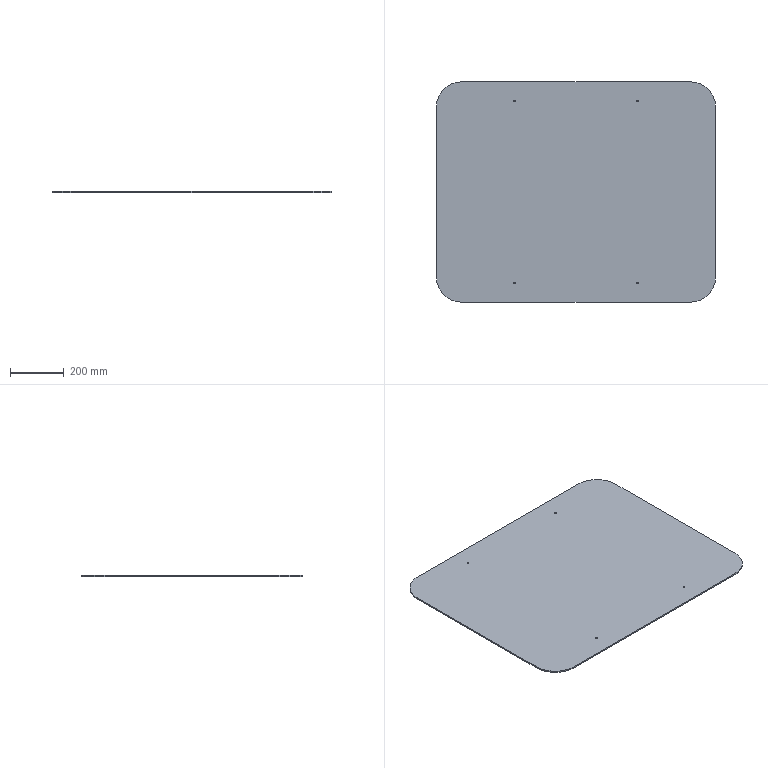Part | NX | features BREP 1 | 1 solid | 14 faces | box 1040 x 820 x 5 mm | volume 4224601 mm3 | cylinder 8 | plane 6 | commonest cylinder face diameters 6.5 x4 190 x4
STEP:
#1=CARTESIAN_POINT('',(232.75,338.5,-5.));
#2=VERTEX_POINT('',#1);
#3=CARTESIAN_POINT('',(229.5,338.5,-5.));
#4=DIRECTION('',(0.,0.,-1.));
#5=DIRECTION('',(1.,0.,0.));
#6=AXIS2_PLACEMENT_3D('',#3,#4,#5);
#7=CIRCLE('',#6,3.25);
#8=EDGE_CURVE('',#2,#2,#7,.T.);
#9=ORIENTED_EDGE('',*,*,#8,.T.);
#10=EDGE_LOOP('',(#9));
#11=FACE_BOUND('',#10,.T.);
#12=CARTESIAN_POINT('',(226.25,338.5,0.));
#13=VERTEX_POINT('',#12);
#14=CARTESIAN_POINT('',(229.5,338.5,0.));
#15=DIRECTION('',(0.,0.,-1.));
#16=DIRECTION('',(-1.,0.,0.));
#17=AXIS2_PLACEMENT_3D('',#14,#15,#16);
#18=CIRCLE('',#17,3.25);
#19=EDGE_CURVE('',#13,#13,#18,.T.);
#20=ORIENTED_EDGE('',*,*,#19,.F.);
#21=EDGE_LOOP('',(#20));
#22=FACE_BOUND('',#21,.T.);
#23=CARTESIAN_POINT('',(229.5,338.5,5.));
#24=DIRECTION('',(0.,0.,-1.));
#25=DIRECTION('',(-1.,0.,0.));
#26=AXIS2_PLACEMENT_3D('',#23,#24,#25);
#27=CYLINDRICAL_SURFACE('',#26,3.25);
#28=ADVANCED_FACE('',(#11,#22),#27,.F.);
#29=CARTESIAN_POINT('',(-232.75,338.5,-5.));
#30=VERTEX_POINT('',#29);
#31=CARTESIAN_POINT('',(-229.5,338.5,-5.));
#32=DIRECTION('',(0.,0.,-1.));
#33=DIRECTION('',(-1.,0.,0.));
#34=AXIS2_PLACEMENT_3D('',#31,#32,#33);
#35=CIRCLE('',#34,3.25);
#36=EDGE_CURVE('',#30,#30,#35,.T.);
#37=ORIENTED_EDGE('',*,*,#36,.T.);
#38=EDGE_LOOP('',(#37));
#39=FACE_BOUND('',#38,.T.);
#40=CARTESIAN_POINT('',(-232.75,338.5,0.));
#41=VERTEX_POINT('',#40);
#42=CARTESIAN_POINT('',(-229.5,338.5,0.));
#43=DIRECTION('',(0.,0.,-1.));
#44=DIRECTION('',(-1.,0.,0.));
#45=AXIS2_PLACEMENT_3D('',#42,#43,#44);
#46=CIRCLE('',#45,3.25);
#47=EDGE_CURVE('',#41,#41,#46,.T.);
#48=ORIENTED_EDGE('',*,*,#47,.F.);
#49=EDGE_LOOP('',(#48));
#50=FACE_BOUND('',#49,.T.);
#51=CARTESIAN_POINT('',(-229.5,338.5,5.));
#52=DIRECTION('',(0.,0.,-1.));
#53=DIRECTION('',(-1.,0.,0.));
#54=AXIS2_PLACEMENT_3D('',#51,#52,#53);
#55=CYLINDRICAL_SURFACE('',#54,3.25);
#56=ADVANCED_FACE('',(#39,#50),#55,.F.);
#57=CARTESIAN_POINT('',(-226.25,-338.5,-5.));
#58=VERTEX_POINT('',#57);
#59=CARTESIAN_POINT('',(-229.5,-338.5,-5.));
#60=DIRECTION('',(0.,0.,-1.));
#61=DIRECTION('',(1.,0.,0.));
#62=AXIS2_PLACEMENT_3D('',#59,#60,#61);
#63=CIRCLE('',#62,3.25);
#64=EDGE_CURVE('',#58,#58,#63,.T.);
#65=ORIENTED_EDGE('',*,*,#64,.T.);
#66=EDGE_LOOP('',(#65));
#67=FACE_BOUND('',#66,.T.);
#68=CARTESIAN_POINT('',(-232.75,-338.5,0.));
#69=VERTEX_POINT('',#68);
#70=CARTESIAN_POINT('',(-229.5,-338.5,0.));
#71=DIRECTION('',(0.,0.,-1.));
#72=DIRECTION('',(-1.,0.,0.));
#73=AXIS2_PLACEMENT_3D('',#70,#71,#72);
#74=CIRCLE('',#73,3.25);
#75=EDGE_CURVE('',#69,#69,#74,.T.);
#76=ORIENTED_EDGE('',*,*,#75,.F.);
#77=EDGE_LOOP('',(#76));
#78=FACE_BOUND('',#77,.T.);
#79=CARTESIAN_POINT('',(-229.5,-338.5,5.));
#80=DIRECTION('',(0.,0.,-1.));
#81=DIRECTION('',(-1.,0.,0.));
#82=AXIS2_PLACEMENT_3D('',#79,#80,#81);
#83=CYLINDRICAL_SURFACE('',#82,3.25);
#84=ADVANCED_FACE('',(#67,#78),#83,.F.);
#85=CARTESIAN_POINT('',(226.25,-338.5,-5.));
#86=VERTEX_POINT('',#85);
#87=CARTESIAN_POINT('',(229.5,-338.5,-5.));
#88=DIRECTION('',(0.,0.,-1.));
#89=DIRECTION('',(-1.,0.,0.));
#90=AXIS2_PLACEMENT_3D('',#87,#88,#89);
#91=CIRCLE('',#90,3.25);
#92=EDGE_CURVE('',#86,#86,#91,.T.);
#93=ORIENTED_EDGE('',*,*,#92,.T.);
#94=EDGE_LOOP('',(#93));
#95=FACE_BOUND('',#94,.T.);
#96=CARTESIAN_POINT('',(226.25,-338.5,0.));
#97=VERTEX_POINT('',#96);
#98=CARTESIAN_POINT('',(229.5,-338.5,0.));
#99=DIRECTION('',(0.,0.,-1.));
#100=DIRECTION('',(-1.,0.,0.));
#101=AXIS2_PLACEMENT_3D('',#98,#99,#100);
#102=CIRCLE('',#101,3.25);
#103=EDGE_CURVE('',#97,#97,#102,.T.);
#104=ORIENTED_EDGE('',*,*,#103,.F.);
#105=EDGE_LOOP('',(#104));
#106=FACE_BOUND('',#105,.T.);
#107=CARTESIAN_POINT('',(229.5,-338.5,5.));
#108=DIRECTION('',(0.,0.,-1.));
#109=DIRECTION('',(-1.,0.,0.));
#110=AXIS2_PLACEMENT_3D('',#107,#108,#109);
#111=CYLINDRICAL_SURFACE('',#110,3.25);
#112=ADVANCED_FACE('',(#95,#106),#111,.F.);
#113=CARTESIAN_POINT('',(-425.,410.,0.));
#114=VERTEX_POINT('',#113);
#115=CARTESIAN_POINT('',(-520.,315.,0.));
#116=VERTEX_POINT('',#115);
#117=CARTESIAN_POINT('',(-425.,315.,0.));
#118=DIRECTION('',(0.,0.,1.));
#119=DIRECTION('',(-1.,0.,0.));
#120=AXIS2_PLACEMENT_3D('',#117,#118,#119);
#121=CIRCLE('',#120,95.);
#122=EDGE_CURVE('',#114,#116,#121,.T.);
#123=ORIENTED_EDGE('',*,*,#122,.F.);
#124=CARTESIAN_POINT('',(-425.,410.,-5.));
#125=VERTEX_POINT('',#124);
#126=CARTESIAN_POINT('',(-425.,410.,-5.));
#127=DIRECTION('',(0.,0.,1.));
#128=VECTOR('',#127,1000.);
#129=LINE('',#126,#128);
#130=EDGE_CURVE('',#125,#114,#129,.T.);
#131=ORIENTED_EDGE('',*,*,#130,.F.);
#132=CARTESIAN_POINT('',(-520.,315.,-5.));
#133=VERTEX_POINT('',#132);
#134=CARTESIAN_POINT('',(-425.,315.,-5.));
#135=DIRECTION('',(0.,0.,1.));
#136=DIRECTION('',(-1.,0.,0.));
#137=AXIS2_PLACEMENT_3D('',#134,#135,#136);
#138=CIRCLE('',#137,95.);
#139=EDGE_CURVE('',#125,#133,#138,.T.);
#140=ORIENTED_EDGE('',*,*,#139,.T.);
#141=CARTESIAN_POINT('',(-520.,315.,-5.));
#142=DIRECTION('',(0.,0.,1.));
#143=VECTOR('',#142,1000.);
#144=LINE('',#141,#143);
#145=EDGE_CURVE('',#133,#116,#144,.T.);
#146=ORIENTED_EDGE('',*,*,#145,.T.);
#147=EDGE_LOOP('',(#123,#131,#140,#146));
#148=FACE_BOUND('',#147,.T.);
#149=CARTESIAN_POINT('',(-425.,315.,-5.));
#150=DIRECTION('',(0.,0.,1.));
#151=DIRECTION('',(1.,0.,0.));
#152=AXIS2_PLACEMENT_3D('',#149,#150,#151);
#153=CYLINDRICAL_SURFACE('',#152,95.);
#154=ADVANCED_FACE('',(#148),#153,.T.);
#155=CARTESIAN_POINT('',(425.,410.,0.));
#156=VERTEX_POINT('',#155);
#157=CARTESIAN_POINT('',(-425.,410.,0.));
#158=DIRECTION('',(-1.,0.,0.));
#159=VECTOR('',#158,1000.);
#160=LINE('',#157,#159);
#161=EDGE_CURVE('',#156,#114,#160,.T.);
#162=ORIENTED_EDGE('',*,*,#161,.F.);
#163=CARTESIAN_POINT('',(425.,410.,-5.));
#164=VERTEX_POINT('',#163);
#165=CARTESIAN_POINT('',(425.,410.,-5.));
#166=DIRECTION('',(0.,0.,1.));
#167=VECTOR('',#166,1000.);
#168=LINE('',#165,#167);
#169=EDGE_CURVE('',#164,#156,#168,.T.);
#170=ORIENTED_EDGE('',*,*,#169,.F.);
#171=CARTESIAN_POINT('',(-425.,410.,-5.));
#172=DIRECTION('',(-1.,0.,0.));
#173=VECTOR('',#172,1000.);
#174=LINE('',#171,#173);
#175=EDGE_CURVE('',#164,#125,#174,.T.);
#176=ORIENTED_EDGE('',*,*,#175,.T.);
#177=ORIENTED_EDGE('',*,*,#130,.T.);
#178=EDGE_LOOP('',(#162,#170,#176,#177));
#179=FACE_BOUND('',#178,.T.);
#180=CARTESIAN_POINT('',(-425.,410.,-5.));
#181=DIRECTION('',(0.,1.,0.));
#182=DIRECTION('',(-1.,0.,0.));
#183=AXIS2_PLACEMENT_3D('',#180,#181,#182);
#184=PLANE('',#183);
#185=ADVANCED_FACE('',(#179),#184,.T.);
#186=CARTESIAN_POINT('',(520.,315.,0.));
#187=VERTEX_POINT('',#186);
#188=CARTESIAN_POINT('',(425.,315.,0.));
#189=DIRECTION('',(0.,0.,1.));
#190=DIRECTION('',(-1.,0.,0.));
#191=AXIS2_PLACEMENT_3D('',#188,#189,#190);
#192=CIRCLE('',#191,95.);
#193=EDGE_CURVE('',#187,#156,#192,.T.);
#194=ORIENTED_EDGE('',*,*,#193,.F.);
#195=CARTESIAN_POINT('',(520.,315.,-5.));
#196=VERTEX_POINT('',#195);
#197=CARTESIAN_POINT('',(520.,315.,-5.));
#198=DIRECTION('',(0.,0.,1.));
#199=VECTOR('',#198,1000.);
#200=LINE('',#197,#199);
#201=EDGE_CURVE('',#196,#187,#200,.T.);
#202=ORIENTED_EDGE('',*,*,#201,.F.);
#203=CARTESIAN_POINT('',(425.,315.,-5.));
#204=DIRECTION('',(0.,0.,1.));
#205=DIRECTION('',(-1.,0.,0.));
#206=AXIS2_PLACEMENT_3D('',#203,#204,#205);
#207=CIRCLE('',#206,95.);
#208=EDGE_CURVE('',#196,#164,#207,.T.);
#209=ORIENTED_EDGE('',*,*,#208,.T.);
#210=ORIENTED_EDGE('',*,*,#169,.T.);
#211=EDGE_LOOP('',(#194,#202,#209,#210));
#212=FACE_BOUND('',#211,.T.);
#213=CARTESIAN_POINT('',(425.,315.,-5.));
#214=DIRECTION('',(0.,0.,1.));
#215=DIRECTION('',(1.,0.,0.));
#216=AXIS2_PLACEMENT_3D('',#213,#214,#215);
#217=CYLINDRICAL_SURFACE('',#216,95.);
#218=ADVANCED_FACE('',(#212),#217,.T.);
#219=CARTESIAN_POINT('',(520.,-315.,0.));
#220=VERTEX_POINT('',#219);
#221=CARTESIAN_POINT('',(520.,-315.,0.));
#222=DIRECTION('',(0.,1.,0.));
#223=VECTOR('',#222,1000.);
#224=LINE('',#221,#223);
#225=EDGE_CURVE('',#220,#187,#224,.T.);
#226=ORIENTED_EDGE('',*,*,#225,.F.);
#227=CARTESIAN_POINT('',(520.,-315.,-5.));
#228=VERTEX_POINT('',#227);
#229=CARTESIAN_POINT('',(520.,-315.,-5.));
#230=DIRECTION('',(0.,0.,1.));
#231=VECTOR('',#230,1000.);
#232=LINE('',#229,#231);
#233=EDGE_CURVE('',#228,#220,#232,.T.);
#234=ORIENTED_EDGE('',*,*,#233,.F.);
#235=CARTESIAN_POINT('',(520.,-315.,-5.));
#236=DIRECTION('',(0.,1.,0.));
#237=VECTOR('',#236,1000.);
#238=LINE('',#235,#237);
#239=EDGE_CURVE('',#228,#196,#238,.T.);
#240=ORIENTED_EDGE('',*,*,#239,.T.);
#241=ORIENTED_EDGE('',*,*,#201,.T.);
#242=EDGE_LOOP('',(#226,#234,#240,#241));
#243=FACE_BOUND('',#242,.T.);
#244=CARTESIAN_POINT('',(520.,-315.,-5.));
#245=DIRECTION('',(1.,0.,0.));
#246=DIRECTION('',(0.,0.,-1.));
#247=AXIS2_PLACEMENT_3D('',#244,#245,#246);
#248=PLANE('',#247);
#249=ADVANCED_FACE('',(#243),#248,.T.);
#250=CARTESIAN_POINT('',(425.,-410.,0.));
#251=VERTEX_POINT('',#250);
#252=CARTESIAN_POINT('',(425.,-315.,0.));
#253=DIRECTION('',(0.,0.,1.));
#254=DIRECTION('',(-1.,0.,0.));
#255=AXIS2_PLACEMENT_3D('',#252,#253,#254);
#256=CIRCLE('',#255,95.);
#257=EDGE_CURVE('',#251,#220,#256,.T.);
#258=ORIENTED_EDGE('',*,*,#257,.F.);
#259=CARTESIAN_POINT('',(425.,-410.,-5.));
#260=VERTEX_POINT('',#259);
#261=CARTESIAN_POINT('',(425.,-410.,-5.));
#262=DIRECTION('',(0.,0.,1.));
#263=VECTOR('',#262,1000.);
#264=LINE('',#261,#263);
#265=EDGE_CURVE('',#260,#251,#264,.T.);
#266=ORIENTED_EDGE('',*,*,#265,.F.);
#267=CARTESIAN_POINT('',(425.,-315.,-5.));
#268=DIRECTION('',(0.,0.,1.));
#269=DIRECTION('',(-1.,0.,0.));
#270=AXIS2_PLACEMENT_3D('',#267,#268,#269);
#271=CIRCLE('',#270,95.);
#272=EDGE_CURVE('',#260,#228,#271,.T.);
#273=ORIENTED_EDGE('',*,*,#272,.T.);
#274=ORIENTED_EDGE('',*,*,#233,.T.);
#275=EDGE_LOOP('',(#258,#266,#273,#274));
#276=FACE_BOUND('',#275,.T.);
#277=CARTESIAN_POINT('',(425.,-315.,-5.));
#278=DIRECTION('',(0.,0.,1.));
#279=DIRECTION('',(1.,0.,0.));
#280=AXIS2_PLACEMENT_3D('',#277,#278,#279);
#281=CYLINDRICAL_SURFACE('',#280,95.);
#282=ADVANCED_FACE('',(#276),#281,.T.);
#283=CARTESIAN_POINT('',(-425.,-410.,0.));
#284=VERTEX_POINT('',#283);
#285=CARTESIAN_POINT('',(-425.,-410.,0.));
#286=DIRECTION('',(1.,0.,0.));
#287=VECTOR('',#286,1000.);
#288=LINE('',#285,#287);
#289=EDGE_CURVE('',#284,#251,#288,.T.);
#290=ORIENTED_EDGE('',*,*,#289,.F.);
#291=CARTESIAN_POINT('',(-425.,-410.,-5.));
#292=VERTEX_POINT('',#291);
#293=CARTESIAN_POINT('',(-425.,-410.,-5.));
#294=DIRECTION('',(0.,0.,1.));
#295=VECTOR('',#294,1000.);
#296=LINE('',#293,#295);
#297=EDGE_CURVE('',#292,#284,#296,.T.);
#298=ORIENTED_EDGE('',*,*,#297,.F.);
#299=CARTESIAN_POINT('',(-425.,-410.,-5.));
#300=DIRECTION('',(1.,0.,0.));
#301=VECTOR('',#300,1000.);
#302=LINE('',#299,#301);
#303=EDGE_CURVE('',#292,#260,#302,.T.);
#304=ORIENTED_EDGE('',*,*,#303,.T.);
#305=ORIENTED_EDGE('',*,*,#265,.T.);
#306=EDGE_LOOP('',(#290,#298,#304,#305));
#307=FACE_BOUND('',#306,.T.);
#308=CARTESIAN_POINT('',(-425.,-410.,-5.));
#309=DIRECTION('',(0.,-1.,0.));
#310=DIRECTION('',(1.,0.,0.));
#311=AXIS2_PLACEMENT_3D('',#308,#309,#310);
#312=PLANE('',#311);
#313=ADVANCED_FACE('',(#307),#312,.T.);
#314=CARTESIAN_POINT('',(-520.,-315.,0.));
#315=VERTEX_POINT('',#314);
#316=CARTESIAN_POINT('',(-425.,-315.,0.));
#317=DIRECTION('',(0.,0.,1.));
#318=DIRECTION('',(-1.,0.,0.));
#319=AXIS2_PLACEMENT_3D('',#316,#317,#318);
#320=CIRCLE('',#319,95.);
#321=EDGE_CURVE('',#315,#284,#320,.T.);
#322=ORIENTED_EDGE('',*,*,#321,.F.);
#323=CARTESIAN_POINT('',(-520.,-315.,-5.));
#324=VERTEX_POINT('',#323);
#325=CARTESIAN_POINT('',(-520.,-315.,-5.));
#326=DIRECTION('',(0.,0.,1.));
#327=VECTOR('',#326,1000.);
#328=LINE('',#325,#327);
#329=EDGE_CURVE('',#324,#315,#328,.T.);
#330=ORIENTED_EDGE('',*,*,#329,.F.);
#331=CARTESIAN_POINT('',(-425.,-315.,-5.));
#332=DIRECTION('',(0.,0.,1.));
#333=DIRECTION('',(-1.,0.,0.));
#334=AXIS2_PLACEMENT_3D('',#331,#332,#333);
#335=CIRCLE('',#334,95.);
#336=EDGE_CURVE('',#324,#292,#335,.T.);
#337=ORIENTED_EDGE('',*,*,#336,.T.);
#338=ORIENTED_EDGE('',*,*,#297,.T.);
#339=EDGE_LOOP('',(#322,#330,#337,#338));
#340=FACE_BOUND('',#339,.T.);
#341=CARTESIAN_POINT('',(-425.,-315.,-5.));
#342=DIRECTION('',(0.,0.,1.));
#343=DIRECTION('',(1.,0.,0.));
#344=AXIS2_PLACEMENT_3D('',#341,#342,#343);
#345=CYLINDRICAL_SURFACE('',#344,95.);
#346=ADVANCED_FACE('',(#340),#345,.T.);
#347=CARTESIAN_POINT('',(-520.,-315.,0.));
#348=DIRECTION('',(0.,-1.,0.));
#349=VECTOR('',#348,1000.);
#350=LINE('',#347,#349);
#351=EDGE_CURVE('',#116,#315,#350,.T.);
#352=ORIENTED_EDGE('',*,*,#351,.F.);
#353=ORIENTED_EDGE('',*,*,#145,.F.);
#354=CARTESIAN_POINT('',(-520.,-315.,-5.));
#355=DIRECTION('',(0.,-1.,0.));
#356=VECTOR('',#355,1000.);
#357=LINE('',#354,#356);
#358=EDGE_CURVE('',#133,#324,#357,.T.);
#359=ORIENTED_EDGE('',*,*,#358,.T.);
#360=ORIENTED_EDGE('',*,*,#329,.T.);
#361=EDGE_LOOP('',(#352,#353,#359,#360));
#362=FACE_BOUND('',#361,.T.);
#363=CARTESIAN_POINT('',(-520.,-315.,-5.));
#364=DIRECTION('',(-1.,0.,0.));
#365=DIRECTION('',(0.,-1.,0.));
#366=AXIS2_PLACEMENT_3D('',#363,#364,#365);
#367=PLANE('',#366);
#368=ADVANCED_FACE('',(#362),#367,.T.);
#369=ORIENTED_EDGE('',*,*,#8,.F.);
#370=EDGE_LOOP('',(#369));
#371=FACE_BOUND('',#370,.T.);
#372=ORIENTED_EDGE('',*,*,#36,.F.);
#373=EDGE_LOOP('',(#372));
#374=FACE_BOUND('',#373,.T.);
#375=ORIENTED_EDGE('',*,*,#64,.F.);
#376=EDGE_LOOP('',(#375));
#377=FACE_BOUND('',#376,.T.);
#378=ORIENTED_EDGE('',*,*,#92,.F.);
#379=EDGE_LOOP('',(#378));
#380=FACE_BOUND('',#379,.T.);
#381=ORIENTED_EDGE('',*,*,#139,.F.);
#382=ORIENTED_EDGE('',*,*,#175,.F.);
#383=ORIENTED_EDGE('',*,*,#208,.F.);
#384=ORIENTED_EDGE('',*,*,#239,.F.);
#385=ORIENTED_EDGE('',*,*,#272,.F.);
#386=ORIENTED_EDGE('',*,*,#303,.F.);
#387=ORIENTED_EDGE('',*,*,#336,.F.);
#388=ORIENTED_EDGE('',*,*,#358,.F.);
#389=EDGE_LOOP('',(#381,#382,#383,#384,#385,#386,#387,#388));
#390=FACE_BOUND('',#389,.T.);
#391=CARTESIAN_POINT('',(-425.,315.,-5.));
#392=DIRECTION('',(0.,0.,-1.));
#393=DIRECTION('',(-1.,0.,0.));
#394=AXIS2_PLACEMENT_3D('',#391,#392,#393);
#395=PLANE('',#394);
#396=ADVANCED_FACE('',(#371,#374,#377,#380,#390),#395,.T.);
#397=ORIENTED_EDGE('',*,*,#19,.T.);
#398=EDGE_LOOP('',(#397));
#399=FACE_BOUND('',#398,.T.);
#400=ORIENTED_EDGE('',*,*,#47,.T.);
#401=EDGE_LOOP('',(#400));
#402=FACE_BOUND('',#401,.T.);
#403=ORIENTED_EDGE('',*,*,#75,.T.);
#404=EDGE_LOOP('',(#403));
#405=FACE_BOUND('',#404,.T.);
#406=ORIENTED_EDGE('',*,*,#103,.T.);
#407=EDGE_LOOP('',(#406));
#408=FACE_BOUND('',#407,.T.);
#409=ORIENTED_EDGE('',*,*,#122,.T.);
#410=ORIENTED_EDGE('',*,*,#351,.T.);
#411=ORIENTED_EDGE('',*,*,#321,.T.);
#412=ORIENTED_EDGE('',*,*,#289,.T.);
#413=ORIENTED_EDGE('',*,*,#257,.T.);
#414=ORIENTED_EDGE('',*,*,#225,.T.);
#415=ORIENTED_EDGE('',*,*,#193,.T.);
#416=ORIENTED_EDGE('',*,*,#161,.T.);
#417=EDGE_LOOP('',(#409,#410,#411,#412,#413,#414,#415,#416));
#418=FACE_BOUND('',#417,.T.);
#419=CARTESIAN_POINT('',(-425.,315.,0.));
#420=DIRECTION('',(0.,0.,-1.));
#421=DIRECTION('',(-1.,0.,0.));
#422=AXIS2_PLACEMENT_3D('',#419,#420,#421);
#423=PLANE('',#422);
#424=ADVANCED_FACE('',(#399,#402,#405,#408,#418),#423,.F.);
#425=CLOSED_SHELL('',(#28,#56,#84,#112,#154,#185,#218,#249,#282,#313,#346,#368,#396,#424));
#426=MANIFOLD_SOLID_BREP('',#425);
#427=(LENGTH_UNIT()NAMED_UNIT(*)SI_UNIT(.MILLI.,.METRE.));
#428=UNCERTAINTY_MEASURE_WITH_UNIT(LENGTH_MEASURE(0.00001),#427,'','');
#429=(NAMED_UNIT(*)PLANE_ANGLE_UNIT()SI_UNIT($,.RADIAN.));
#430=(NAMED_UNIT(*)SI_UNIT($,.STERADIAN.)SOLID_ANGLE_UNIT());
#431=(GEOMETRIC_REPRESENTATION_CONTEXT(3)GLOBAL_UNCERTAINTY_ASSIGNED_CONTEXT((#428))GLOBAL_UNIT_ASSIGNED_CONTEXT((#427,#429,#430))REPRESENTATION_CONTEXT('',''));
#432=ADVANCED_BREP_SHAPE_REPRESENTATION('',(#426),#431);